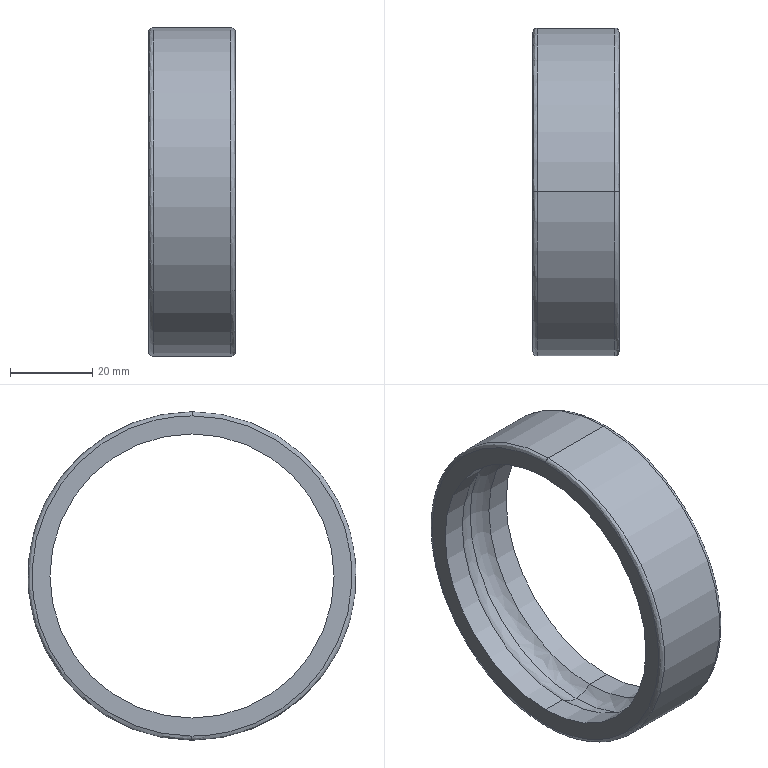Part | STEP file | Outer Ring | 1 solid | 16 faces | box 21 x 80 x 80 mm | volume 23803 mm3 | spline 8 | cylinder 6 | plane 2 | commonest cylinder face diameters 69.2 x4 80 x2
STEP:
#1=CARTESIAN_POINT('',(0.,0.,39.));
#2=VERTEX_POINT('',#1);
#3=CARTESIAN_POINT('',(0.,0.,-39.));
#4=VERTEX_POINT('',#3);
#5=CARTESIAN_POINT('',(0.,0.,39.));
#6=CARTESIAN_POINT('',(0.,-78.,39.));
#7=CARTESIAN_POINT('',(0.,-78.,-39.));
#8=CARTESIAN_POINT('',(0.,0.,-39.));
#9=(BOUNDED_CURVE()B_SPLINE_CURVE(3,(#5,#6,#7,#8),.UNSPECIFIED.,.F.,.F.)B_SPLINE_CURVE_WITH_KNOTS((4,4),(0.,0.5),.UNSPECIFIED.)CURVE()GEOMETRIC_REPRESENTATION_ITEM()RATIONAL_B_SPLINE_CURVE((1.,0.3333,0.3333,1.))REPRESENTATION_ITEM(''));
#10=EDGE_CURVE('',#2,#4,#9,.T.);
#11=ORIENTED_EDGE('',*,*,#10,.T.);
#12=CARTESIAN_POINT('',(1.,0.,-40.));
#13=VERTEX_POINT('',#12);
#14=CARTESIAN_POINT('',(1.,0.,-39.));
#15=DIRECTION('',(0.,-1.,0.));
#16=DIRECTION('',(0.,0.,-1.));
#17=AXIS2_PLACEMENT_3D('',#14,#15,#16);
#18=CIRCLE('',#17,1.);
#19=EDGE_CURVE('',#4,#13,#18,.T.);
#20=ORIENTED_EDGE('',*,*,#19,.T.);
#21=CARTESIAN_POINT('',(1.,0.,40.));
#22=VERTEX_POINT('',#21);
#23=CARTESIAN_POINT('',(1.,0.,0.));
#24=DIRECTION('',(1.,0.,0.));
#25=DIRECTION('',(0.,0.,-1.));
#26=AXIS2_PLACEMENT_3D('',#23,#24,#25);
#27=CIRCLE('',#26,40.);
#28=EDGE_CURVE('',#22,#13,#27,.T.);
#29=ORIENTED_EDGE('',*,*,#28,.F.);
#30=CARTESIAN_POINT('',(1.,0.,39.));
#31=DIRECTION('',(0.,1.,0.));
#32=DIRECTION('',(0.,0.,1.));
#33=AXIS2_PLACEMENT_3D('',#30,#31,#32);
#34=CIRCLE('',#33,1.);
#35=EDGE_CURVE('',#2,#22,#34,.T.);
#36=ORIENTED_EDGE('',*,*,#35,.F.);
#37=EDGE_LOOP('',(#11,#20,#29,#36));
#38=FACE_OUTER_BOUND('',#37,.T.);
#39=CARTESIAN_POINT('',(0.,0.,-39.));
#40=CARTESIAN_POINT('',(0.,-78.,-39.));
#41=CARTESIAN_POINT('',(0.,-78.,39.));
#42=CARTESIAN_POINT('',(0.,0.,39.));
#43=CARTESIAN_POINT('',(0.,0.,-39.586));
#44=CARTESIAN_POINT('',(0.,-79.172,-39.586));
#45=CARTESIAN_POINT('',(0.,-79.172,39.586));
#46=CARTESIAN_POINT('',(0.,0.,39.586));
#47=CARTESIAN_POINT('',(0.4142,0.,-40.));
#48=CARTESIAN_POINT('',(0.4142,-80.,-40.));
#49=CARTESIAN_POINT('',(0.4142,-80.,40.));
#50=CARTESIAN_POINT('',(0.4142,0.,40.));
#51=CARTESIAN_POINT('',(1.,0.,-40.));
#52=CARTESIAN_POINT('',(1.,-80.,-40.));
#53=CARTESIAN_POINT('',(1.,-80.,40.));
#54=CARTESIAN_POINT('',(1.,0.,40.));
#55=(BOUNDED_SURFACE()B_SPLINE_SURFACE(3,3,((#39,#40,#41,#42),(#43,#44,#45,#46),(#47,#48,#49,#50),(#51,#52,#53,#54)),.UNSPECIFIED.,.F.,.F.,.F.)B_SPLINE_SURFACE_WITH_KNOTS((4,4),(4,4),(0.,1.),(0.,1.),.UNSPECIFIED.)GEOMETRIC_REPRESENTATION_ITEM()RATIONAL_B_SPLINE_SURFACE(((1.,0.3333,0.3333,1.),(0.8047,0.2682,0.2682,0.8047),(0.8047,0.2682,0.2682,0.8047),(1.,0.3333,0.3333,1.)))REPRESENTATION_ITEM('')SURFACE());
#56=ADVANCED_FACE('',(#38),#55,.T.);
#57=CARTESIAN_POINT('',(21.,0.,-39.));
#58=VERTEX_POINT('',#57);
#59=CARTESIAN_POINT('',(21.,0.,39.));
#60=VERTEX_POINT('',#59);
#61=CARTESIAN_POINT('',(21.,0.,-39.));
#62=CARTESIAN_POINT('',(21.,-78.,-39.));
#63=CARTESIAN_POINT('',(21.,-78.,39.));
#64=CARTESIAN_POINT('',(21.,0.,39.));
#65=(BOUNDED_CURVE()B_SPLINE_CURVE(3,(#61,#62,#63,#64),.UNSPECIFIED.,.F.,.F.)B_SPLINE_CURVE_WITH_KNOTS((4,4),(0.,0.5),.UNSPECIFIED.)CURVE()GEOMETRIC_REPRESENTATION_ITEM()RATIONAL_B_SPLINE_CURVE((1.,0.3333,0.3333,1.))REPRESENTATION_ITEM(''));
#66=EDGE_CURVE('',#58,#60,#65,.T.);
#67=ORIENTED_EDGE('',*,*,#66,.T.);
#68=CARTESIAN_POINT('',(20.,0.,40.));
#69=VERTEX_POINT('',#68);
#70=CARTESIAN_POINT('',(20.,0.,39.));
#71=DIRECTION('',(0.,-1.,0.));
#72=DIRECTION('',(0.,0.,1.));
#73=AXIS2_PLACEMENT_3D('',#70,#71,#72);
#74=CIRCLE('',#73,1.);
#75=EDGE_CURVE('',#60,#69,#74,.T.);
#76=ORIENTED_EDGE('',*,*,#75,.T.);
#77=CARTESIAN_POINT('',(20.,0.,-40.));
#78=VERTEX_POINT('',#77);
#79=CARTESIAN_POINT('',(20.,0.,0.));
#80=DIRECTION('',(-1.,0.,0.));
#81=DIRECTION('',(0.,0.,-1.));
#82=AXIS2_PLACEMENT_3D('',#79,#80,#81);
#83=CIRCLE('',#82,40.);
#84=EDGE_CURVE('',#78,#69,#83,.T.);
#85=ORIENTED_EDGE('',*,*,#84,.F.);
#86=CARTESIAN_POINT('',(20.,0.,-39.));
#87=DIRECTION('',(0.,1.,0.));
#88=DIRECTION('',(0.,0.,-1.));
#89=AXIS2_PLACEMENT_3D('',#86,#87,#88);
#90=CIRCLE('',#89,1.);
#91=EDGE_CURVE('',#58,#78,#90,.T.);
#92=ORIENTED_EDGE('',*,*,#91,.F.);
#93=EDGE_LOOP('',(#67,#76,#85,#92));
#94=FACE_OUTER_BOUND('',#93,.T.);
#95=CARTESIAN_POINT('',(21.,0.,39.));
#96=CARTESIAN_POINT('',(21.,-78.,39.));
#97=CARTESIAN_POINT('',(21.,-78.,-39.));
#98=CARTESIAN_POINT('',(21.,0.,-39.));
#99=CARTESIAN_POINT('',(21.,0.,39.586));
#100=CARTESIAN_POINT('',(21.,-79.172,39.586));
#101=CARTESIAN_POINT('',(21.,-79.172,-39.586));
#102=CARTESIAN_POINT('',(21.,0.,-39.586));
#103=CARTESIAN_POINT('',(20.586,0.,40.));
#104=CARTESIAN_POINT('',(20.586,-80.,40.));
#105=CARTESIAN_POINT('',(20.586,-80.,-40.));
#106=CARTESIAN_POINT('',(20.586,0.,-40.));
#107=CARTESIAN_POINT('',(20.,0.,40.));
#108=CARTESIAN_POINT('',(20.,-80.,40.));
#109=CARTESIAN_POINT('',(20.,-80.,-40.));
#110=CARTESIAN_POINT('',(20.,0.,-40.));
#111=(BOUNDED_SURFACE()B_SPLINE_SURFACE(3,3,((#95,#96,#97,#98),(#99,#100,#101,#102),(#103,#104,#105,#106),(#107,#108,#109,#110)),.UNSPECIFIED.,.F.,.F.,.F.)B_SPLINE_SURFACE_WITH_KNOTS((4,4),(4,4),(0.,1.),(0.,1.),.UNSPECIFIED.)GEOMETRIC_REPRESENTATION_ITEM()RATIONAL_B_SPLINE_SURFACE(((1.,0.3333,0.3333,1.),(0.8047,0.2682,0.2682,0.8047),(0.8047,0.2682,0.2682,0.8047),(1.,0.3333,0.3333,1.)))REPRESENTATION_ITEM('')SURFACE());
#112=ADVANCED_FACE('',(#94),#111,.T.);
#113=CARTESIAN_POINT('',(5.908,0.,34.6));
#114=VERTEX_POINT('',#113);
#115=CARTESIAN_POINT('',(5.908,0.,-34.6));
#116=VERTEX_POINT('',#115);
#117=CARTESIAN_POINT('',(5.908,0.,0.));
#118=DIRECTION('',(-1.,0.,0.));
#119=DIRECTION('',(0.,0.,-1.));
#120=AXIS2_PLACEMENT_3D('',#117,#118,#119);
#121=CIRCLE('',#120,34.6);
#122=EDGE_CURVE('',#114,#116,#121,.T.);
#123=ORIENTED_EDGE('',*,*,#122,.T.);
#124=CARTESIAN_POINT('',(10.5,0.,-36.5));
#125=VERTEX_POINT('',#124);
#126=CARTESIAN_POINT('',(10.5,0.,-30.));
#127=DIRECTION('',(0.,-1.,0.));
#128=DIRECTION('',(0.,0.,-1.));
#129=AXIS2_PLACEMENT_3D('',#126,#127,#128);
#130=CIRCLE('',#129,6.5);
#131=EDGE_CURVE('',#116,#125,#130,.T.);
#132=ORIENTED_EDGE('',*,*,#131,.T.);
#133=CARTESIAN_POINT('',(10.5,0.,36.5));
#134=VERTEX_POINT('',#133);
#135=CARTESIAN_POINT('',(10.5,0.,0.));
#136=DIRECTION('',(-1.,0.,0.));
#137=DIRECTION('',(0.,0.,1.));
#138=AXIS2_PLACEMENT_3D('',#135,#136,#137);
#139=CIRCLE('',#138,36.5);
#140=EDGE_CURVE('',#134,#125,#139,.T.);
#141=ORIENTED_EDGE('',*,*,#140,.F.);
#142=CARTESIAN_POINT('',(10.5,0.,30.));
#143=DIRECTION('',(0.,1.,0.));
#144=DIRECTION('',(0.,0.,1.));
#145=AXIS2_PLACEMENT_3D('',#142,#143,#144);
#146=CIRCLE('',#145,6.5);
#147=EDGE_CURVE('',#114,#134,#146,.T.);
#148=ORIENTED_EDGE('',*,*,#147,.F.);
#149=EDGE_LOOP('',(#123,#132,#141,#148));
#150=FACE_OUTER_BOUND('',#149,.T.);
#151=CARTESIAN_POINT('',(5.908,0.,34.6));
#152=CARTESIAN_POINT('',(5.908,69.2,34.6));
#153=CARTESIAN_POINT('',(5.908,69.2,-34.6));
#154=CARTESIAN_POINT('',(5.908,0.,-34.6));
#155=CARTESIAN_POINT('',(7.143,0.,35.833));
#156=CARTESIAN_POINT('',(7.143,71.666,35.833));
#157=CARTESIAN_POINT('',(7.143,71.666,-35.833));
#158=CARTESIAN_POINT('',(7.143,0.,-35.833));
#159=CARTESIAN_POINT('',(8.755,0.,36.5));
#160=CARTESIAN_POINT('',(8.755,73.,36.5));
#161=CARTESIAN_POINT('',(8.755,73.,-36.5));
#162=CARTESIAN_POINT('',(8.755,0.,-36.5));
#163=CARTESIAN_POINT('',(10.5,0.,36.5));
#164=CARTESIAN_POINT('',(10.5,73.,36.5));
#165=CARTESIAN_POINT('',(10.5,73.,-36.5));
#166=CARTESIAN_POINT('',(10.5,0.,-36.5));
#167=(BOUNDED_SURFACE()B_SPLINE_SURFACE(3,3,((#151,#152,#153,#154),(#155,#156,#157,#158),(#159,#160,#161,#162),(#163,#164,#165,#166)),.UNSPECIFIED.,.F.,.F.,.F.)B_SPLINE_SURFACE_WITH_KNOTS((4,4),(4,4),(0.,1.),(0.,1.),.UNSPECIFIED.)GEOMETRIC_REPRESENTATION_ITEM()RATIONAL_B_SPLINE_SURFACE(((1.,0.3333,0.3333,1.),(0.9494,0.3165,0.3165,0.9494),(0.9494,0.3165,0.3165,0.9494),(1.,0.3333,0.3333,1.)))REPRESENTATION_ITEM('')SURFACE());
#168=ADVANCED_FACE('',(#150),#167,.F.);
#169=ORIENTED_EDGE('',*,*,#140,.T.);
#170=CARTESIAN_POINT('',(15.092,0.,-34.6));
#171=VERTEX_POINT('',#170);
#172=CARTESIAN_POINT('',(10.5,0.,-30.));
#173=DIRECTION('',(0.,-1.,0.));
#174=DIRECTION('',(0.,0.,-1.));
#175=AXIS2_PLACEMENT_3D('',#172,#173,#174);
#176=CIRCLE('',#175,6.5);
#177=EDGE_CURVE('',#125,#171,#176,.T.);
#178=ORIENTED_EDGE('',*,*,#177,.T.);
#179=CARTESIAN_POINT('',(15.092,0.,34.6));
#180=VERTEX_POINT('',#179);
#181=CARTESIAN_POINT('',(15.092,0.,0.));
#182=DIRECTION('',(1.,0.,0.));
#183=DIRECTION('',(0.,0.,-1.));
#184=AXIS2_PLACEMENT_3D('',#181,#182,#183);
#185=CIRCLE('',#184,34.6);
#186=EDGE_CURVE('',#171,#180,#185,.T.);
#187=ORIENTED_EDGE('',*,*,#186,.T.);
#188=CARTESIAN_POINT('',(10.5,0.,30.));
#189=DIRECTION('',(0.,1.,0.));
#190=DIRECTION('',(0.,0.,1.));
#191=AXIS2_PLACEMENT_3D('',#188,#189,#190);
#192=CIRCLE('',#191,6.5);
#193=EDGE_CURVE('',#134,#180,#192,.T.);
#194=ORIENTED_EDGE('',*,*,#193,.F.);
#195=EDGE_LOOP('',(#169,#178,#187,#194));
#196=FACE_OUTER_BOUND('',#195,.T.);
#197=CARTESIAN_POINT('',(10.5,0.,36.5));
#198=CARTESIAN_POINT('',(10.5,73.,36.5));
#199=CARTESIAN_POINT('',(10.5,73.,-36.5));
#200=CARTESIAN_POINT('',(10.5,0.,-36.5));
#201=CARTESIAN_POINT('',(12.245,0.,36.5));
#202=CARTESIAN_POINT('',(12.245,73.,36.5));
#203=CARTESIAN_POINT('',(12.245,73.,-36.5));
#204=CARTESIAN_POINT('',(12.245,0.,-36.5));
#205=CARTESIAN_POINT('',(13.857,0.,35.833));
#206=CARTESIAN_POINT('',(13.857,71.666,35.833));
#207=CARTESIAN_POINT('',(13.857,71.666,-35.833));
#208=CARTESIAN_POINT('',(13.857,0.,-35.833));
#209=CARTESIAN_POINT('',(15.092,0.,34.6));
#210=CARTESIAN_POINT('',(15.092,69.2,34.6));
#211=CARTESIAN_POINT('',(15.092,69.2,-34.6));
#212=CARTESIAN_POINT('',(15.092,0.,-34.6));
#213=(BOUNDED_SURFACE()B_SPLINE_SURFACE(3,3,((#197,#198,#199,#200),(#201,#202,#203,#204),(#205,#206,#207,#208),(#209,#210,#211,#212)),.UNSPECIFIED.,.F.,.F.,.F.)B_SPLINE_SURFACE_WITH_KNOTS((4,4),(4,4),(0.,1.),(0.,1.),.UNSPECIFIED.)GEOMETRIC_REPRESENTATION_ITEM()RATIONAL_B_SPLINE_SURFACE(((1.,0.3333,0.3333,1.),(0.9494,0.3165,0.3165,0.9494),(0.9494,0.3165,0.3165,0.9494),(1.,0.3333,0.3333,1.)))REPRESENTATION_ITEM('')SURFACE());
#214=ADVANCED_FACE('',(#196),#213,.F.);
#215=CARTESIAN_POINT('',(1.,0.,0.));
#216=DIRECTION('',(1.,0.,0.));
#217=DIRECTION('',(0.,0.,-1.));
#218=AXIS2_PLACEMENT_3D('',#215,#216,#217);
#219=CIRCLE('',#218,40.);
#220=EDGE_CURVE('',#13,#22,#219,.T.);
#221=ORIENTED_EDGE('',*,*,#220,.T.);
#222=CARTESIAN_POINT('',(-0.8903,0.,40.));
#223=DIRECTION('',(1.,0.,0.));
#224=VECTOR('',#223,1000.);
#225=LINE('',#222,#224);
#226=EDGE_CURVE('',#22,#69,#225,.T.);
#227=ORIENTED_EDGE('',*,*,#226,.T.);
#228=CARTESIAN_POINT('',(20.,0.,0.));
#229=DIRECTION('',(-1.,0.,0.));
#230=DIRECTION('',(0.,0.,-1.));
#231=AXIS2_PLACEMENT_3D('',#228,#229,#230);
#232=CIRCLE('',#231,40.);
#233=EDGE_CURVE('',#69,#78,#232,.T.);
#234=ORIENTED_EDGE('',*,*,#233,.T.);
#235=CARTESIAN_POINT('',(-0.8903,0.,-40.));
#236=DIRECTION('',(1.,0.,0.));
#237=VECTOR('',#236,1000.);
#238=LINE('',#235,#237);
#239=EDGE_CURVE('',#13,#78,#238,.T.);
#240=ORIENTED_EDGE('',*,*,#239,.F.);
#241=EDGE_LOOP('',(#221,#227,#234,#240));
#242=FACE_OUTER_BOUND('',#241,.T.);
#243=CARTESIAN_POINT('',(-0.8903,0.,0.));
#244=DIRECTION('',(1.,0.,0.));
#245=DIRECTION('',(0.,0.,-1.));
#246=AXIS2_PLACEMENT_3D('',#243,#244,#245);
#247=CYLINDRICAL_SURFACE('',#246,40.);
#248=ADVANCED_FACE('',(#242),#247,.T.);
#249=CARTESIAN_POINT('',(0.,0.,34.6));
#250=VERTEX_POINT('',#249);
#251=CARTESIAN_POINT('',(0.,0.,-34.6));
#252=VERTEX_POINT('',#251);
#253=CARTESIAN_POINT('',(0.,0.,0.));
#254=DIRECTION('',(1.,0.,0.));
#255=DIRECTION('',(0.,0.,-1.));
#256=AXIS2_PLACEMENT_3D('',#253,#254,#255);
#257=CIRCLE('',#256,34.6);
#258=EDGE_CURVE('',#250,#252,#257,.T.);
#259=ORIENTED_EDGE('',*,*,#258,.F.);
#260=CARTESIAN_POINT('',(-0.8903,0.,34.6));
#261=DIRECTION('',(1.,0.,0.));
#262=VECTOR('',#261,1000.);
#263=LINE('',#260,#262);
#264=EDGE_CURVE('',#250,#114,#263,.T.);
#265=ORIENTED_EDGE('',*,*,#264,.T.);
#266=CARTESIAN_POINT('',(5.908,0.,0.));
#267=DIRECTION('',(-1.,0.,0.));
#268=DIRECTION('',(0.,0.,-1.));
#269=AXIS2_PLACEMENT_3D('',#266,#267,#268);
#270=CIRCLE('',#269,34.6);
#271=EDGE_CURVE('',#116,#114,#270,.T.);
#272=ORIENTED_EDGE('',*,*,#271,.F.);
#273=CARTESIAN_POINT('',(-0.8903,0.,-34.6));
#274=DIRECTION('',(1.,0.,0.));
#275=VECTOR('',#274,1000.);
#276=LINE('',#273,#275);
#277=EDGE_CURVE('',#252,#116,#276,.T.);
#278=ORIENTED_EDGE('',*,*,#277,.F.);
#279=EDGE_LOOP('',(#259,#265,#272,#278));
#280=FACE_OUTER_BOUND('',#279,.T.);
#281=CARTESIAN_POINT('',(-0.8903,0.,0.));
#282=DIRECTION('',(1.,0.,0.));
#283=DIRECTION('',(0.,0.,-1.));
#284=AXIS2_PLACEMENT_3D('',#281,#282,#283);
#285=CYLINDRICAL_SURFACE('',#284,34.6);
#286=ADVANCED_FACE('',(#280),#285,.F.);
#287=CARTESIAN_POINT('',(15.092,0.,0.));
#288=DIRECTION('',(1.,0.,0.));
#289=DIRECTION('',(0.,0.,-1.));
#290=AXIS2_PLACEMENT_3D('',#287,#288,#289);
#291=CIRCLE('',#290,34.6);
#292=EDGE_CURVE('',#180,#171,#291,.T.);
#293=ORIENTED_EDGE('',*,*,#292,.F.);
#294=CARTESIAN_POINT('',(21.,0.,34.6));
#295=VERTEX_POINT('',#294);
#296=CARTESIAN_POINT('',(-0.8903,0.,34.6));
#297=DIRECTION('',(1.,0.,0.));
#298=VECTOR('',#297,1000.);
#299=LINE('',#296,#298);
#300=EDGE_CURVE('',#180,#295,#299,.T.);
#301=ORIENTED_EDGE('',*,*,#300,.T.);
#302=CARTESIAN_POINT('',(21.,0.,-34.6));
#303=VERTEX_POINT('',#302);
#304=CARTESIAN_POINT('',(21.,0.,0.));
#305=DIRECTION('',(-1.,0.,0.));
#306=DIRECTION('',(0.,0.,-1.));
#307=AXIS2_PLACEMENT_3D('',#304,#305,#306);
#308=CIRCLE('',#307,34.6);
#309=EDGE_CURVE('',#303,#295,#308,.T.);
#310=ORIENTED_EDGE('',*,*,#309,.F.);
#311=CARTESIAN_POINT('',(-0.8903,0.,-34.6));
#312=DIRECTION('',(1.,0.,0.));
#313=VECTOR('',#312,1000.);
#314=LINE('',#311,#313);
#315=EDGE_CURVE('',#171,#303,#314,.T.);
#316=ORIENTED_EDGE('',*,*,#315,.F.);
#317=EDGE_LOOP('',(#293,#301,#310,#316));
#318=FACE_OUTER_BOUND('',#317,.T.);
#319=CARTESIAN_POINT('',(-0.8903,0.,0.));
#320=DIRECTION('',(1.,0.,0.));
#321=DIRECTION('',(0.,0.,-1.));
#322=AXIS2_PLACEMENT_3D('',#319,#320,#321);
#323=CYLINDRICAL_SURFACE('',#322,34.6);
#324=ADVANCED_FACE('',(#318),#323,.F.);
#325=ORIENTED_EDGE('',*,*,#177,.F.);
#326=CARTESIAN_POINT('',(10.5,0.,0.));
#327=DIRECTION('',(-1.,0.,0.));
#328=DIRECTION('',(0.,0.,1.));
#329=AXIS2_PLACEMENT_3D('',#326,#327,#328);
#330=CIRCLE('',#329,36.5);
#331=EDGE_CURVE('',#125,#134,#330,.T.);
#332=ORIENTED_EDGE('',*,*,#331,.T.);
#333=ORIENTED_EDGE('',*,*,#193,.T.);
#334=ORIENTED_EDGE('',*,*,#292,.T.);
#335=EDGE_LOOP('',(#325,#332,#333,#334));
#336=FACE_OUTER_BOUND('',#335,.T.);
#337=CARTESIAN_POINT('',(10.5,0.,-36.5));
#338=CARTESIAN_POINT('',(10.5,-73.,-36.5));
#339=CARTESIAN_POINT('',(10.5,-73.,36.5));
#340=CARTESIAN_POINT('',(10.5,0.,36.5));
#341=CARTESIAN_POINT('',(12.245,0.,-36.5));
#342=CARTESIAN_POINT('',(12.245,-73.,-36.5));
#343=CARTESIAN_POINT('',(12.245,-73.,36.5));
#344=CARTESIAN_POINT('',(12.245,0.,36.5));
#345=CARTESIAN_POINT('',(13.857,0.,-35.833));
#346=CARTESIAN_POINT('',(13.857,-71.666,-35.833));
#347=CARTESIAN_POINT('',(13.857,-71.666,35.833));
#348=CARTESIAN_POINT('',(13.857,0.,35.833));
#349=CARTESIAN_POINT('',(15.092,0.,-34.6));
#350=CARTESIAN_POINT('',(15.092,-69.2,-34.6));
#351=CARTESIAN_POINT('',(15.092,-69.2,34.6));
#352=CARTESIAN_POINT('',(15.092,0.,34.6));
#353=(BOUNDED_SURFACE()B_SPLINE_SURFACE(3,3,((#337,#338,#339,#340),(#341,#342,#343,#344),(#345,#346,#347,#348),(#349,#350,#351,#352)),.UNSPECIFIED.,.F.,.F.,.F.)B_SPLINE_SURFACE_WITH_KNOTS((4,4),(4,4),(0.,1.),(0.,1.),.UNSPECIFIED.)GEOMETRIC_REPRESENTATION_ITEM()RATIONAL_B_SPLINE_SURFACE(((1.,0.3333,0.3333,1.),(0.9494,0.3165,0.3165,0.9494),(0.9494,0.3165,0.3165,0.9494),(1.,0.3333,0.3333,1.)))REPRESENTATION_ITEM('')SURFACE());
#354=ADVANCED_FACE('',(#336),#353,.F.);
#355=ORIENTED_EDGE('',*,*,#226,.F.);
#356=ORIENTED_EDGE('',*,*,#28,.T.);
#357=ORIENTED_EDGE('',*,*,#239,.T.);
#358=ORIENTED_EDGE('',*,*,#84,.T.);
#359=EDGE_LOOP('',(#355,#356,#357,#358));
#360=FACE_OUTER_BOUND('',#359,.T.);
#361=CARTESIAN_POINT('',(-0.8903,0.,0.));
#362=DIRECTION('',(1.,0.,0.));
#363=DIRECTION('',(0.,0.,-1.));
#364=AXIS2_PLACEMENT_3D('',#361,#362,#363);
#365=CYLINDRICAL_SURFACE('',#364,40.);
#366=ADVANCED_FACE('',(#360),#365,.T.);
#367=ORIENTED_EDGE('',*,*,#19,.F.);
#368=CARTESIAN_POINT('',(0.,0.,-39.));
#369=CARTESIAN_POINT('',(0.,78.,-39.));
#370=CARTESIAN_POINT('',(0.,78.,39.));
#371=CARTESIAN_POINT('',(0.,0.,39.));
#372=(BOUNDED_CURVE()B_SPLINE_CURVE(3,(#368,#369,#370,#371),.UNSPECIFIED.,.F.,.F.)B_SPLINE_CURVE_WITH_KNOTS((4,4),(0.5,1.),.UNSPECIFIED.)CURVE()GEOMETRIC_REPRESENTATION_ITEM()RATIONAL_B_SPLINE_CURVE((1.,0.3333,0.3333,1.))REPRESENTATION_ITEM(''));
#373=EDGE_CURVE('',#4,#2,#372,.T.);
#374=ORIENTED_EDGE('',*,*,#373,.T.);
#375=ORIENTED_EDGE('',*,*,#35,.T.);
#376=ORIENTED_EDGE('',*,*,#220,.F.);
#377=EDGE_LOOP('',(#367,#374,#375,#376));
#378=FACE_OUTER_BOUND('',#377,.T.);
#379=CARTESIAN_POINT('',(0.,0.,39.));
#380=CARTESIAN_POINT('',(0.,78.,39.));
#381=CARTESIAN_POINT('',(0.,78.,-39.));
#382=CARTESIAN_POINT('',(0.,0.,-39.));
#383=CARTESIAN_POINT('',(0.,0.,39.586));
#384=CARTESIAN_POINT('',(0.,79.172,39.586));
#385=CARTESIAN_POINT('',(0.,79.172,-39.586));
#386=CARTESIAN_POINT('',(0.,0.,-39.586));
#387=CARTESIAN_POINT('',(0.4142,0.,40.));
#388=CARTESIAN_POINT('',(0.4142,80.,40.));
#389=CARTESIAN_POINT('',(0.4142,80.,-40.));
#390=CARTESIAN_POINT('',(0.4142,0.,-40.));
#391=CARTESIAN_POINT('',(1.,0.,40.));
#392=CARTESIAN_POINT('',(1.,80.,40.));
#393=CARTESIAN_POINT('',(1.,80.,-40.));
#394=CARTESIAN_POINT('',(1.,0.,-40.));
#395=(BOUNDED_SURFACE()B_SPLINE_SURFACE(3,3,((#379,#380,#381,#382),(#383,#384,#385,#386),(#387,#388,#389,#390),(#391,#392,#393,#394)),.UNSPECIFIED.,.F.,.F.,.F.)B_SPLINE_SURFACE_WITH_KNOTS((4,4),(4,4),(0.,1.),(0.,1.),.UNSPECIFIED.)GEOMETRIC_REPRESENTATION_ITEM()RATIONAL_B_SPLINE_SURFACE(((1.,0.3333,0.3333,1.),(0.8047,0.2682,0.2682,0.8047),(0.8047,0.2682,0.2682,0.8047),(1.,0.3333,0.3333,1.)))REPRESENTATION_ITEM('')SURFACE());
#396=ADVANCED_FACE('',(#378),#395,.T.);
#397=ORIENTED_EDGE('',*,*,#75,.F.);
#398=CARTESIAN_POINT('',(21.,0.,39.));
#399=CARTESIAN_POINT('',(21.,78.,39.));
#400=CARTESIAN_POINT('',(21.,78.,-39.));
#401=CARTESIAN_POINT('',(21.,0.,-39.));
#402=(BOUNDED_CURVE()B_SPLINE_CURVE(3,(#398,#399,#400,#401),.UNSPECIFIED.,.F.,.F.)B_SPLINE_CURVE_WITH_KNOTS((4,4),(0.5,1.),.UNSPECIFIED.)CURVE()GEOMETRIC_REPRESENTATION_ITEM()RATIONAL_B_SPLINE_CURVE((1.,0.3333,0.3333,1.))REPRESENTATION_ITEM(''));
#403=EDGE_CURVE('',#60,#58,#402,.T.);
#404=ORIENTED_EDGE('',*,*,#403,.T.);
#405=ORIENTED_EDGE('',*,*,#91,.T.);
#406=ORIENTED_EDGE('',*,*,#233,.F.);
#407=EDGE_LOOP('',(#397,#404,#405,#406));
#408=FACE_OUTER_BOUND('',#407,.T.);
#409=CARTESIAN_POINT('',(21.,0.,-39.));
#410=CARTESIAN_POINT('',(21.,78.,-39.));
#411=CARTESIAN_POINT('',(21.,78.,39.));
#412=CARTESIAN_POINT('',(21.,0.,39.));
#413=CARTESIAN_POINT('',(21.,0.,-39.586));
#414=CARTESIAN_POINT('',(21.,79.172,-39.586));
#415=CARTESIAN_POINT('',(21.,79.172,39.586));
#416=CARTESIAN_POINT('',(21.,0.,39.586));
#417=CARTESIAN_POINT('',(20.586,0.,-40.));
#418=CARTESIAN_POINT('',(20.586,80.,-40.));
#419=CARTESIAN_POINT('',(20.586,80.,40.));
#420=CARTESIAN_POINT('',(20.586,0.,40.));
#421=CARTESIAN_POINT('',(20.,0.,-40.));
#422=CARTESIAN_POINT('',(20.,80.,-40.));
#423=CARTESIAN_POINT('',(20.,80.,40.));
#424=CARTESIAN_POINT('',(20.,0.,40.));
#425=(BOUNDED_SURFACE()B_SPLINE_SURFACE(3,3,((#409,#410,#411,#412),(#413,#414,#415,#416),(#417,#418,#419,#420),(#421,#422,#423,#424)),.UNSPECIFIED.,.F.,.F.,.F.)B_SPLINE_SURFACE_WITH_KNOTS((4,4),(4,4),(0.,1.),(0.,1.),.UNSPECIFIED.)GEOMETRIC_REPRESENTATION_ITEM()RATIONAL_B_SPLINE_SURFACE(((1.,0.3333,0.3333,1.),(0.8047,0.2682,0.2682,0.8047),(0.8047,0.2682,0.2682,0.8047),(1.,0.3333,0.3333,1.)))REPRESENTATION_ITEM('')SURFACE());
#426=ADVANCED_FACE('',(#408),#425,.T.);
#427=CARTESIAN_POINT('',(0.,0.,0.));
#428=DIRECTION('',(1.,0.,0.));
#429=DIRECTION('',(0.,0.,-1.));
#430=AXIS2_PLACEMENT_3D('',#427,#428,#429);
#431=CIRCLE('',#430,34.6);
#432=EDGE_CURVE('',#252,#250,#431,.T.);
#433=ORIENTED_EDGE('',*,*,#432,.T.);
#434=ORIENTED_EDGE('',*,*,#258,.T.);
#435=EDGE_LOOP('',(#433,#434));
#436=FACE_BOUND('',#435,.T.);
#437=ORIENTED_EDGE('',*,*,#10,.F.);
#438=ORIENTED_EDGE('',*,*,#373,.F.);
#439=EDGE_LOOP('',(#437,#438));
#440=FACE_OUTER_BOUND('',#439,.T.);
#441=CARTESIAN_POINT('',(0.,0.,34.6));
#442=DIRECTION('',(-1.,0.,0.));
#443=DIRECTION('',(0.,0.,1.));
#444=AXIS2_PLACEMENT_3D('',#441,#442,#443);
#445=PLANE('',#444);
#446=ADVANCED_FACE('',(#436,#440),#445,.T.);
#447=ORIENTED_EDGE('',*,*,#309,.T.);
#448=CARTESIAN_POINT('',(21.,0.,0.));
#449=DIRECTION('',(-1.,0.,0.));
#450=DIRECTION('',(0.,0.,-1.));
#451=AXIS2_PLACEMENT_3D('',#448,#449,#450);
#452=CIRCLE('',#451,34.6);
#453=EDGE_CURVE('',#295,#303,#452,.T.);
#454=ORIENTED_EDGE('',*,*,#453,.T.);
#455=EDGE_LOOP('',(#447,#454));
#456=FACE_BOUND('',#455,.T.);
#457=ORIENTED_EDGE('',*,*,#66,.F.);
#458=ORIENTED_EDGE('',*,*,#403,.F.);
#459=EDGE_LOOP('',(#457,#458));
#460=FACE_OUTER_BOUND('',#459,.T.);
#461=CARTESIAN_POINT('',(21.,0.,34.6));
#462=DIRECTION('',(1.,0.,0.));
#463=DIRECTION('',(0.,0.,-1.));
#464=AXIS2_PLACEMENT_3D('',#461,#462,#463);
#465=PLANE('',#464);
#466=ADVANCED_FACE('',(#456,#460),#465,.T.);
#467=ORIENTED_EDGE('',*,*,#264,.F.);
#468=ORIENTED_EDGE('',*,*,#432,.F.);
#469=ORIENTED_EDGE('',*,*,#277,.T.);
#470=ORIENTED_EDGE('',*,*,#122,.F.);
#471=EDGE_LOOP('',(#467,#468,#469,#470));
#472=FACE_OUTER_BOUND('',#471,.T.);
#473=CARTESIAN_POINT('',(-0.8903,0.,0.));
#474=DIRECTION('',(1.,0.,0.));
#475=DIRECTION('',(0.,0.,-1.));
#476=AXIS2_PLACEMENT_3D('',#473,#474,#475);
#477=CYLINDRICAL_SURFACE('',#476,34.6);
#478=ADVANCED_FACE('',(#472),#477,.F.);
#479=ORIENTED_EDGE('',*,*,#300,.F.);
#480=ORIENTED_EDGE('',*,*,#186,.F.);
#481=ORIENTED_EDGE('',*,*,#315,.T.);
#482=ORIENTED_EDGE('',*,*,#453,.F.);
#483=EDGE_LOOP('',(#479,#480,#481,#482));
#484=FACE_OUTER_BOUND('',#483,.T.);
#485=CARTESIAN_POINT('',(-0.8903,0.,0.));
#486=DIRECTION('',(1.,0.,0.));
#487=DIRECTION('',(0.,0.,-1.));
#488=AXIS2_PLACEMENT_3D('',#485,#486,#487);
#489=CYLINDRICAL_SURFACE('',#488,34.6);
#490=ADVANCED_FACE('',(#484),#489,.F.);
#491=ORIENTED_EDGE('',*,*,#131,.F.);
#492=ORIENTED_EDGE('',*,*,#271,.T.);
#493=ORIENTED_EDGE('',*,*,#147,.T.);
#494=ORIENTED_EDGE('',*,*,#331,.F.);
#495=EDGE_LOOP('',(#491,#492,#493,#494));
#496=FACE_OUTER_BOUND('',#495,.T.);
#497=CARTESIAN_POINT('',(5.908,0.,-34.6));
#498=CARTESIAN_POINT('',(5.908,-69.2,-34.6));
#499=CARTESIAN_POINT('',(5.908,-69.2,34.6));
#500=CARTESIAN_POINT('',(5.908,0.,34.6));
#501=CARTESIAN_POINT('',(7.143,0.,-35.833));
#502=CARTESIAN_POINT('',(7.143,-71.666,-35.833));
#503=CARTESIAN_POINT('',(7.143,-71.666,35.833));
#504=CARTESIAN_POINT('',(7.143,0.,35.833));
#505=CARTESIAN_POINT('',(8.755,0.,-36.5));
#506=CARTESIAN_POINT('',(8.755,-73.,-36.5));
#507=CARTESIAN_POINT('',(8.755,-73.,36.5));
#508=CARTESIAN_POINT('',(8.755,0.,36.5));
#509=CARTESIAN_POINT('',(10.5,0.,-36.5));
#510=CARTESIAN_POINT('',(10.5,-73.,-36.5));
#511=CARTESIAN_POINT('',(10.5,-73.,36.5));
#512=CARTESIAN_POINT('',(10.5,0.,36.5));
#513=(BOUNDED_SURFACE()B_SPLINE_SURFACE(3,3,((#497,#498,#499,#500),(#501,#502,#503,#504),(#505,#506,#507,#508),(#509,#510,#511,#512)),.UNSPECIFIED.,.F.,.F.,.F.)B_SPLINE_SURFACE_WITH_KNOTS((4,4),(4,4),(0.,1.),(0.,1.),.UNSPECIFIED.)GEOMETRIC_REPRESENTATION_ITEM()RATIONAL_B_SPLINE_SURFACE(((1.,0.3333,0.3333,1.),(0.9494,0.3165,0.3165,0.9494),(0.9494,0.3165,0.3165,0.9494),(1.,0.3333,0.3333,1.)))REPRESENTATION_ITEM('')SURFACE());
#514=ADVANCED_FACE('',(#496),#513,.F.);
#515=CLOSED_SHELL('',(#56,#112,#168,#214,#248,#286,#324,#354,#366,#396,#426,#446,#466,#478,#490,#514));
#516=MANIFOLD_SOLID_BREP('',#515);
#517=CARTESIAN_POINT('',(0.,0.,0.));
#518=DIRECTION('',(0.,0.,1.));
#519=DIRECTION('',(1.,0.,0.));
#520=AXIS2_PLACEMENT_3D('',#517,#518,#519);
#521=(LENGTH_UNIT()NAMED_UNIT(*)SI_UNIT(.MILLI.,.METRE.));
#522=UNCERTAINTY_MEASURE_WITH_UNIT(LENGTH_MEASURE(0.00001),#521,'','');
#523=(NAMED_UNIT(*)PLANE_ANGLE_UNIT()SI_UNIT($,.RADIAN.));
#524=(NAMED_UNIT(*)SI_UNIT($,.STERADIAN.)SOLID_ANGLE_UNIT());
#525=(GEOMETRIC_REPRESENTATION_CONTEXT(3)GLOBAL_UNCERTAINTY_ASSIGNED_CONTEXT((#522))GLOBAL_UNIT_ASSIGNED_CONTEXT((#521,#523,#524))REPRESENTATION_CONTEXT('',''));
#526=ADVANCED_BREP_SHAPE_REPRESENTATION('',(#516,#520),#525);